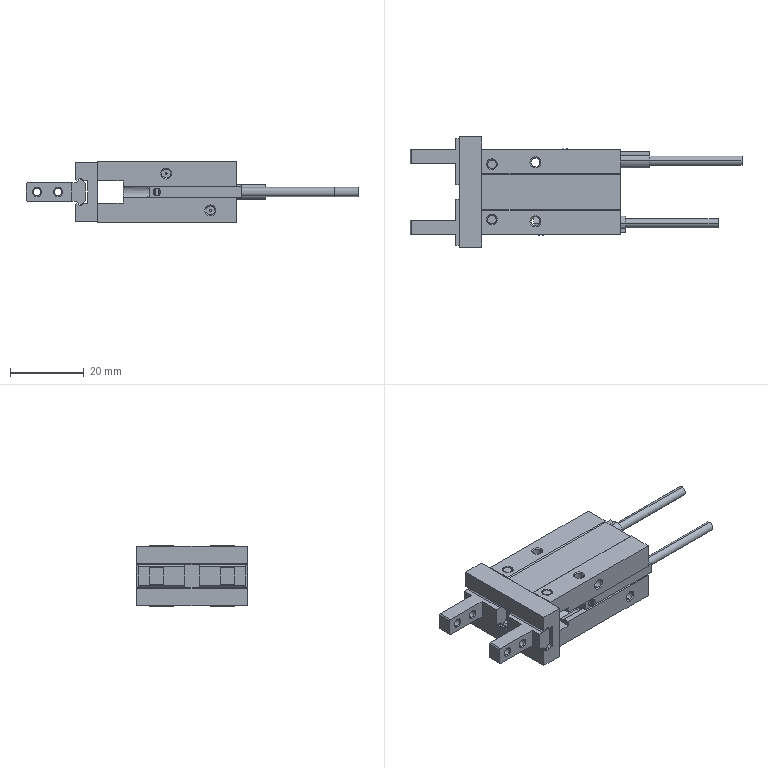Part | SolidWorks | 5 solids | 279 faces | box 90 x 30 x 16.5 mm | volume 15703 mm3 | plane 124 | cylinder 79 | cone 76 | commonest cylinder face diameters 2.459 x20 0.4 x8 2.013 x8 3.02 x8 0.5 x7 4 x6